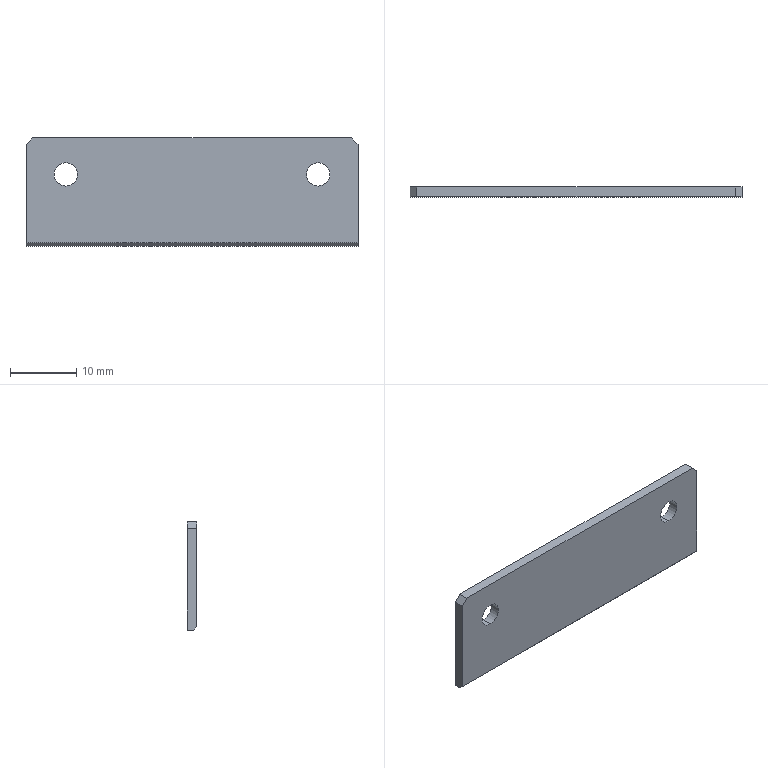Part | SolidWorks | features Chamfer 2, Extrusion 1, ICE 1 | 1 solid | 13 faces | box 50 x 1.5 x 16.3 mm | volume 1186 mm3 | plane 9 | cylinder 4 | commonest cylinder face diameters 3.5 x4
STEP:
#1=CARTESIAN_POINT('',(19.,0.,0.9));
#2=VERTEX_POINT('',#1);
#3=CARTESIAN_POINT('',(19.,0.,4.4));
#4=VERTEX_POINT('',#3);
#5=CARTESIAN_POINT('',(19.,0.,2.65));
#6=DIRECTION('',(0.,1.,0.));
#7=DIRECTION('',(0.,0.,1.));
#8=AXIS2_PLACEMENT_3D('',#5,#6,#7);
#9=CIRCLE('',#8,1.75);
#10=EDGE_CURVE('',#2,#4,#9,.T.);
#11=ORIENTED_EDGE('',*,*,#10,.F.);
#12=CARTESIAN_POINT('',(19.,1.5,0.9));
#13=VERTEX_POINT('',#12);
#14=CARTESIAN_POINT('',(19.,-8.5,0.9));
#15=DIRECTION('',(0.,1.,0.));
#16=VECTOR('',#15,1000.);
#17=LINE('',#14,#16);
#18=EDGE_CURVE('',#2,#13,#17,.T.);
#19=ORIENTED_EDGE('',*,*,#18,.T.);
#20=CARTESIAN_POINT('',(19.,1.5,4.4));
#21=VERTEX_POINT('',#20);
#22=CARTESIAN_POINT('',(19.,1.5,2.65));
#23=DIRECTION('',(0.,1.,0.));
#24=DIRECTION('',(0.,0.,-1.));
#25=AXIS2_PLACEMENT_3D('',#22,#23,#24);
#26=CIRCLE('',#25,1.75);
#27=EDGE_CURVE('',#13,#21,#26,.T.);
#28=ORIENTED_EDGE('',*,*,#27,.T.);
#29=CARTESIAN_POINT('',(19.,-8.5,4.4));
#30=DIRECTION('',(0.,1.,0.));
#31=VECTOR('',#30,1000.);
#32=LINE('',#29,#31);
#33=EDGE_CURVE('',#4,#21,#32,.T.);
#34=ORIENTED_EDGE('',*,*,#33,.F.);
#35=EDGE_LOOP('',(#11,#19,#28,#34));
#36=FACE_OUTER_BOUND('',#35,.T.);
#37=CARTESIAN_POINT('',(19.,-8.5,2.65));
#38=DIRECTION('',(0.,1.,0.));
#39=DIRECTION('',(0.,0.,1.));
#40=AXIS2_PLACEMENT_3D('',#37,#38,#39);
#41=CYLINDRICAL_SURFACE('',#40,1.75);
#42=ADVANCED_FACE('',(#36),#41,.F.);
#43=CARTESIAN_POINT('',(-19.,0.,0.9));
#44=VERTEX_POINT('',#43);
#45=CARTESIAN_POINT('',(-19.,0.,4.4));
#46=VERTEX_POINT('',#45);
#47=CARTESIAN_POINT('',(-19.,0.,2.65));
#48=DIRECTION('',(0.,1.,0.));
#49=DIRECTION('',(0.,0.,1.));
#50=AXIS2_PLACEMENT_3D('',#47,#48,#49);
#51=CIRCLE('',#50,1.75);
#52=EDGE_CURVE('',#44,#46,#51,.T.);
#53=ORIENTED_EDGE('',*,*,#52,.F.);
#54=CARTESIAN_POINT('',(-19.,1.5,0.9));
#55=VERTEX_POINT('',#54);
#56=CARTESIAN_POINT('',(-19.,-8.5,0.9));
#57=DIRECTION('',(0.,1.,0.));
#58=VECTOR('',#57,1000.);
#59=LINE('',#56,#58);
#60=EDGE_CURVE('',#44,#55,#59,.T.);
#61=ORIENTED_EDGE('',*,*,#60,.T.);
#62=CARTESIAN_POINT('',(-19.,1.5,4.4));
#63=VERTEX_POINT('',#62);
#64=CARTESIAN_POINT('',(-19.,1.5,2.65));
#65=DIRECTION('',(0.,1.,0.));
#66=DIRECTION('',(0.,0.,1.));
#67=AXIS2_PLACEMENT_3D('',#64,#65,#66);
#68=CIRCLE('',#67,1.75);
#69=EDGE_CURVE('',#55,#63,#68,.T.);
#70=ORIENTED_EDGE('',*,*,#69,.T.);
#71=CARTESIAN_POINT('',(-19.,-8.5,4.4));
#72=DIRECTION('',(0.,1.,0.));
#73=VECTOR('',#72,1000.);
#74=LINE('',#71,#73);
#75=EDGE_CURVE('',#46,#63,#74,.T.);
#76=ORIENTED_EDGE('',*,*,#75,.F.);
#77=EDGE_LOOP('',(#53,#61,#70,#76));
#78=FACE_OUTER_BOUND('',#77,.T.);
#79=CARTESIAN_POINT('',(-19.,-8.5,2.65));
#80=DIRECTION('',(0.,1.,0.));
#81=DIRECTION('',(0.,0.,1.));
#82=AXIS2_PLACEMENT_3D('',#79,#80,#81);
#83=CYLINDRICAL_SURFACE('',#82,1.75);
#84=ADVANCED_FACE('',(#78),#83,.F.);
#85=CARTESIAN_POINT('',(25.,0.,7.15));
#86=VERTEX_POINT('',#85);
#87=CARTESIAN_POINT('',(25.,0.,-7.65));
#88=VERTEX_POINT('',#87);
#89=CARTESIAN_POINT('',(25.,0.,-8.15));
#90=DIRECTION('',(0.,0.,-1.));
#91=VECTOR('',#90,1000.);
#92=LINE('',#89,#91);
#93=EDGE_CURVE('',#86,#88,#92,.T.);
#94=ORIENTED_EDGE('',*,*,#93,.T.);
#95=CARTESIAN_POINT('',(25.,0.5,-8.15));
#96=VERTEX_POINT('',#95);
#97=CARTESIAN_POINT('',(25.,0.5,-8.15));
#98=DIRECTION('',(0.,0.7071,-0.7071));
#99=VECTOR('',#98,1000.);
#100=LINE('',#97,#99);
#101=EDGE_CURVE('',#88,#96,#100,.T.);
#102=ORIENTED_EDGE('',*,*,#101,.T.);
#103=CARTESIAN_POINT('',(25.,1.5,-8.15));
#104=VERTEX_POINT('',#103);
#105=CARTESIAN_POINT('',(25.,1.5,-8.15));
#106=DIRECTION('',(0.,-1.,0.));
#107=VECTOR('',#106,1000.);
#108=LINE('',#105,#107);
#109=EDGE_CURVE('',#104,#96,#108,.T.);
#110=ORIENTED_EDGE('',*,*,#109,.F.);
#111=CARTESIAN_POINT('',(25.,1.5,7.15));
#112=VERTEX_POINT('',#111);
#113=CARTESIAN_POINT('',(25.,1.5,-8.15));
#114=DIRECTION('',(0.,0.,-1.));
#115=VECTOR('',#114,1000.);
#116=LINE('',#113,#115);
#117=EDGE_CURVE('',#112,#104,#116,.T.);
#118=ORIENTED_EDGE('',*,*,#117,.F.);
#119=CARTESIAN_POINT('',(25.,1.5,7.15));
#120=DIRECTION('',(0.,-1.,0.));
#121=VECTOR('',#120,1000.);
#122=LINE('',#119,#121);
#123=EDGE_CURVE('',#112,#86,#122,.T.);
#124=ORIENTED_EDGE('',*,*,#123,.T.);
#125=EDGE_LOOP('',(#94,#102,#110,#118,#124));
#126=FACE_OUTER_BOUND('',#125,.T.);
#127=CARTESIAN_POINT('',(25.,1.5,-8.15));
#128=DIRECTION('',(-1.,0.,0.));
#129=DIRECTION('',(0.,0.,1.));
#130=AXIS2_PLACEMENT_3D('',#127,#128,#129);
#131=PLANE('',#130);
#132=ADVANCED_FACE('',(#126),#131,.F.);
#133=ORIENTED_EDGE('',*,*,#109,.T.);
#134=CARTESIAN_POINT('',(-25.,0.5,-8.15));
#135=VERTEX_POINT('',#134);
#136=CARTESIAN_POINT('',(-25.,0.5,-8.15));
#137=DIRECTION('',(-1.,0.,0.));
#138=VECTOR('',#137,1000.);
#139=LINE('',#136,#138);
#140=EDGE_CURVE('',#96,#135,#139,.T.);
#141=ORIENTED_EDGE('',*,*,#140,.T.);
#142=CARTESIAN_POINT('',(-25.,1.5,-8.15));
#143=VERTEX_POINT('',#142);
#144=CARTESIAN_POINT('',(-25.,1.5,-8.15));
#145=DIRECTION('',(0.,-1.,0.));
#146=VECTOR('',#145,1000.);
#147=LINE('',#144,#146);
#148=EDGE_CURVE('',#143,#135,#147,.T.);
#149=ORIENTED_EDGE('',*,*,#148,.F.);
#150=CARTESIAN_POINT('',(-25.,1.5,-8.15));
#151=DIRECTION('',(-1.,0.,0.));
#152=VECTOR('',#151,1000.);
#153=LINE('',#150,#152);
#154=EDGE_CURVE('',#104,#143,#153,.T.);
#155=ORIENTED_EDGE('',*,*,#154,.F.);
#156=EDGE_LOOP('',(#133,#141,#149,#155));
#157=FACE_OUTER_BOUND('',#156,.T.);
#158=CARTESIAN_POINT('',(-25.,1.5,-8.15));
#159=DIRECTION('',(0.,0.,1.));
#160=DIRECTION('',(1.,0.,0.));
#161=AXIS2_PLACEMENT_3D('',#158,#159,#160);
#162=PLANE('',#161);
#163=ADVANCED_FACE('',(#157),#162,.F.);
#164=ORIENTED_EDGE('',*,*,#148,.T.);
#165=CARTESIAN_POINT('',(-25.,0.,-7.65));
#166=VERTEX_POINT('',#165);
#167=CARTESIAN_POINT('',(-25.,0.5,-8.15));
#168=DIRECTION('',(0.,-0.7071,0.7071));
#169=VECTOR('',#168,1000.);
#170=LINE('',#167,#169);
#171=EDGE_CURVE('',#135,#166,#170,.T.);
#172=ORIENTED_EDGE('',*,*,#171,.T.);
#173=CARTESIAN_POINT('',(-25.,0.,7.15));
#174=VERTEX_POINT('',#173);
#175=CARTESIAN_POINT('',(-25.,0.,-8.15));
#176=DIRECTION('',(0.,0.,1.));
#177=VECTOR('',#176,1000.);
#178=LINE('',#175,#177);
#179=EDGE_CURVE('',#166,#174,#178,.T.);
#180=ORIENTED_EDGE('',*,*,#179,.T.);
#181=CARTESIAN_POINT('',(-25.,1.5,7.15));
#182=VERTEX_POINT('',#181);
#183=CARTESIAN_POINT('',(-25.,1.5,7.15));
#184=DIRECTION('',(0.,1.,0.));
#185=VECTOR('',#184,1000.);
#186=LINE('',#183,#185);
#187=EDGE_CURVE('',#174,#182,#186,.T.);
#188=ORIENTED_EDGE('',*,*,#187,.T.);
#189=CARTESIAN_POINT('',(-25.,1.5,-8.15));
#190=DIRECTION('',(0.,0.,1.));
#191=VECTOR('',#190,1000.);
#192=LINE('',#189,#191);
#193=EDGE_CURVE('',#143,#182,#192,.T.);
#194=ORIENTED_EDGE('',*,*,#193,.F.);
#195=EDGE_LOOP('',(#164,#172,#180,#188,#194));
#196=FACE_OUTER_BOUND('',#195,.T.);
#197=CARTESIAN_POINT('',(-25.,1.5,-8.15));
#198=DIRECTION('',(1.,0.,0.));
#199=DIRECTION('',(0.,0.,-1.));
#200=AXIS2_PLACEMENT_3D('',#197,#198,#199);
#201=PLANE('',#200);
#202=ADVANCED_FACE('',(#196),#201,.F.);
#203=CARTESIAN_POINT('',(-24.,0.,8.15));
#204=VERTEX_POINT('',#203);
#205=CARTESIAN_POINT('',(24.,0.,8.15));
#206=VERTEX_POINT('',#205);
#207=CARTESIAN_POINT('',(-25.,0.,8.15));
#208=DIRECTION('',(1.,0.,0.));
#209=VECTOR('',#208,1000.);
#210=LINE('',#207,#209);
#211=EDGE_CURVE('',#204,#206,#210,.T.);
#212=ORIENTED_EDGE('',*,*,#211,.T.);
#213=CARTESIAN_POINT('',(24.,1.5,8.15));
#214=VERTEX_POINT('',#213);
#215=CARTESIAN_POINT('',(24.,1.5,8.15));
#216=DIRECTION('',(0.,1.,0.));
#217=VECTOR('',#216,1000.);
#218=LINE('',#215,#217);
#219=EDGE_CURVE('',#206,#214,#218,.T.);
#220=ORIENTED_EDGE('',*,*,#219,.T.);
#221=CARTESIAN_POINT('',(-24.,1.5,8.15));
#222=VERTEX_POINT('',#221);
#223=CARTESIAN_POINT('',(-25.,1.5,8.15));
#224=DIRECTION('',(1.,0.,0.));
#225=VECTOR('',#224,1000.);
#226=LINE('',#223,#225);
#227=EDGE_CURVE('',#222,#214,#226,.T.);
#228=ORIENTED_EDGE('',*,*,#227,.F.);
#229=CARTESIAN_POINT('',(-24.,1.5,8.15));
#230=DIRECTION('',(0.,-1.,0.));
#231=VECTOR('',#230,1000.);
#232=LINE('',#229,#231);
#233=EDGE_CURVE('',#222,#204,#232,.T.);
#234=ORIENTED_EDGE('',*,*,#233,.T.);
#235=EDGE_LOOP('',(#212,#220,#228,#234));
#236=FACE_OUTER_BOUND('',#235,.T.);
#237=CARTESIAN_POINT('',(-25.,1.5,8.15));
#238=DIRECTION('',(0.,0.,-1.));
#239=DIRECTION('',(-1.,0.,0.));
#240=AXIS2_PLACEMENT_3D('',#237,#238,#239);
#241=PLANE('',#240);
#242=ADVANCED_FACE('',(#236),#241,.F.);
#243=CARTESIAN_POINT('',(19.,1.5,2.65));
#244=DIRECTION('',(0.,1.,0.));
#245=DIRECTION('',(0.,0.,-1.));
#246=AXIS2_PLACEMENT_3D('',#243,#244,#245);
#247=CIRCLE('',#246,1.75);
#248=EDGE_CURVE('',#21,#13,#247,.T.);
#249=ORIENTED_EDGE('',*,*,#248,.F.);
#250=ORIENTED_EDGE('',*,*,#27,.F.);
#251=EDGE_LOOP('',(#249,#250));
#252=FACE_BOUND('',#251,.T.);
#253=CARTESIAN_POINT('',(-19.,1.5,2.65));
#254=DIRECTION('',(0.,1.,0.));
#255=DIRECTION('',(0.,0.,1.));
#256=AXIS2_PLACEMENT_3D('',#253,#254,#255);
#257=CIRCLE('',#256,1.75);
#258=EDGE_CURVE('',#63,#55,#257,.T.);
#259=ORIENTED_EDGE('',*,*,#258,.F.);
#260=ORIENTED_EDGE('',*,*,#69,.F.);
#261=EDGE_LOOP('',(#259,#260));
#262=FACE_BOUND('',#261,.T.);
#263=ORIENTED_EDGE('',*,*,#227,.T.);
#264=CARTESIAN_POINT('',(16.075,1.5,16.075));
#265=DIRECTION('',(0.7071,0.,-0.7071));
#266=VECTOR('',#265,1000.);
#267=LINE('',#264,#266);
#268=EDGE_CURVE('',#214,#112,#267,.T.);
#269=ORIENTED_EDGE('',*,*,#268,.T.);
#270=ORIENTED_EDGE('',*,*,#117,.T.);
#271=ORIENTED_EDGE('',*,*,#154,.T.);
#272=ORIENTED_EDGE('',*,*,#193,.T.);
#273=CARTESIAN_POINT('',(-16.075,1.5,16.075));
#274=DIRECTION('',(0.7071,0.,0.7071));
#275=VECTOR('',#274,1000.);
#276=LINE('',#273,#275);
#277=EDGE_CURVE('',#182,#222,#276,.T.);
#278=ORIENTED_EDGE('',*,*,#277,.T.);
#279=EDGE_LOOP('',(#263,#269,#270,#271,#272,#278));
#280=FACE_OUTER_BOUND('',#279,.T.);
#281=CARTESIAN_POINT('',(0.,1.5,0.));
#282=DIRECTION('',(0.,1.,0.));
#283=DIRECTION('',(0.,0.,1.));
#284=AXIS2_PLACEMENT_3D('',#281,#282,#283);
#285=PLANE('',#284);
#286=ADVANCED_FACE('',(#252,#262,#280),#285,.T.);
#287=CARTESIAN_POINT('',(19.,0.,2.65));
#288=DIRECTION('',(0.,1.,0.));
#289=DIRECTION('',(0.,0.,1.));
#290=AXIS2_PLACEMENT_3D('',#287,#288,#289);
#291=CIRCLE('',#290,1.75);
#292=EDGE_CURVE('',#4,#2,#291,.T.);
#293=ORIENTED_EDGE('',*,*,#292,.T.);
#294=ORIENTED_EDGE('',*,*,#10,.T.);
#295=EDGE_LOOP('',(#293,#294));
#296=FACE_BOUND('',#295,.T.);
#297=CARTESIAN_POINT('',(-19.,0.,2.65));
#298=DIRECTION('',(0.,1.,0.));
#299=DIRECTION('',(0.,0.,1.));
#300=AXIS2_PLACEMENT_3D('',#297,#298,#299);
#301=CIRCLE('',#300,1.75);
#302=EDGE_CURVE('',#46,#44,#301,.T.);
#303=ORIENTED_EDGE('',*,*,#302,.T.);
#304=ORIENTED_EDGE('',*,*,#52,.T.);
#305=EDGE_LOOP('',(#303,#304));
#306=FACE_BOUND('',#305,.T.);
#307=ORIENTED_EDGE('',*,*,#179,.F.);
#308=CARTESIAN_POINT('',(0.,0.,-7.65));
#309=DIRECTION('',(1.,0.,0.));
#310=VECTOR('',#309,1000.);
#311=LINE('',#308,#310);
#312=EDGE_CURVE('',#166,#88,#311,.T.);
#313=ORIENTED_EDGE('',*,*,#312,.T.);
#314=ORIENTED_EDGE('',*,*,#93,.F.);
#315=CARTESIAN_POINT('',(25.,0.,7.15));
#316=DIRECTION('',(-0.7071,0.,0.7071));
#317=VECTOR('',#316,1000.);
#318=LINE('',#315,#317);
#319=EDGE_CURVE('',#86,#206,#318,.T.);
#320=ORIENTED_EDGE('',*,*,#319,.T.);
#321=ORIENTED_EDGE('',*,*,#211,.F.);
#322=CARTESIAN_POINT('',(-24.,0.,8.15));
#323=DIRECTION('',(-0.7071,0.,-0.7071));
#324=VECTOR('',#323,1000.);
#325=LINE('',#322,#324);
#326=EDGE_CURVE('',#204,#174,#325,.T.);
#327=ORIENTED_EDGE('',*,*,#326,.T.);
#328=EDGE_LOOP('',(#307,#313,#314,#320,#321,#327));
#329=FACE_OUTER_BOUND('',#328,.T.);
#330=CARTESIAN_POINT('',(0.,0.,0.));
#331=DIRECTION('',(0.,1.,0.));
#332=DIRECTION('',(0.,0.,1.));
#333=AXIS2_PLACEMENT_3D('',#330,#331,#332);
#334=PLANE('',#333);
#335=ADVANCED_FACE('',(#296,#306,#329),#334,.F.);
#336=ORIENTED_EDGE('',*,*,#60,.F.);
#337=ORIENTED_EDGE('',*,*,#302,.F.);
#338=ORIENTED_EDGE('',*,*,#75,.T.);
#339=ORIENTED_EDGE('',*,*,#258,.T.);
#340=EDGE_LOOP('',(#336,#337,#338,#339));
#341=FACE_OUTER_BOUND('',#340,.T.);
#342=CARTESIAN_POINT('',(-19.,-8.5,2.65));
#343=DIRECTION('',(0.,1.,0.));
#344=DIRECTION('',(0.,0.,1.));
#345=AXIS2_PLACEMENT_3D('',#342,#343,#344);
#346=CYLINDRICAL_SURFACE('',#345,1.75);
#347=ADVANCED_FACE('',(#341),#346,.F.);
#348=ORIENTED_EDGE('',*,*,#18,.F.);
#349=ORIENTED_EDGE('',*,*,#292,.F.);
#350=ORIENTED_EDGE('',*,*,#33,.T.);
#351=ORIENTED_EDGE('',*,*,#248,.T.);
#352=EDGE_LOOP('',(#348,#349,#350,#351));
#353=FACE_OUTER_BOUND('',#352,.T.);
#354=CARTESIAN_POINT('',(19.,-8.5,2.65));
#355=DIRECTION('',(0.,1.,0.));
#356=DIRECTION('',(0.,0.,1.));
#357=AXIS2_PLACEMENT_3D('',#354,#355,#356);
#358=CYLINDRICAL_SURFACE('',#357,1.75);
#359=ADVANCED_FACE('',(#353),#358,.F.);
#360=ORIENTED_EDGE('',*,*,#268,.F.);
#361=ORIENTED_EDGE('',*,*,#219,.F.);
#362=ORIENTED_EDGE('',*,*,#319,.F.);
#363=ORIENTED_EDGE('',*,*,#123,.F.);
#364=EDGE_LOOP('',(#360,#361,#362,#363));
#365=FACE_OUTER_BOUND('',#364,.T.);
#366=CARTESIAN_POINT('',(25.,1.5,7.15));
#367=DIRECTION('',(-0.7071,0.,-0.7071));
#368=DIRECTION('',(0.,-1.,0.));
#369=AXIS2_PLACEMENT_3D('',#366,#367,#368);
#370=PLANE('',#369);
#371=ADVANCED_FACE('',(#365),#370,.F.);
#372=ORIENTED_EDGE('',*,*,#277,.F.);
#373=ORIENTED_EDGE('',*,*,#187,.F.);
#374=ORIENTED_EDGE('',*,*,#326,.F.);
#375=ORIENTED_EDGE('',*,*,#233,.F.);
#376=EDGE_LOOP('',(#372,#373,#374,#375));
#377=FACE_OUTER_BOUND('',#376,.T.);
#378=CARTESIAN_POINT('',(-24.,1.5,8.15));
#379=DIRECTION('',(0.7071,0.,-0.7071));
#380=DIRECTION('',(0.,-1.,0.));
#381=AXIS2_PLACEMENT_3D('',#378,#379,#380);
#382=PLANE('',#381);
#383=ADVANCED_FACE('',(#377),#382,.F.);
#384=ORIENTED_EDGE('',*,*,#101,.F.);
#385=ORIENTED_EDGE('',*,*,#312,.F.);
#386=ORIENTED_EDGE('',*,*,#171,.F.);
#387=ORIENTED_EDGE('',*,*,#140,.F.);
#388=EDGE_LOOP('',(#384,#385,#386,#387));
#389=FACE_OUTER_BOUND('',#388,.T.);
#390=CARTESIAN_POINT('',(-25.,0.5,-8.15));
#391=DIRECTION('',(0.,0.7071,0.7071));
#392=DIRECTION('',(-1.,0.,0.));
#393=AXIS2_PLACEMENT_3D('',#390,#391,#392);
#394=PLANE('',#393);
#395=ADVANCED_FACE('',(#389),#394,.F.);
#396=CLOSED_SHELL('',(#42,#84,#132,#163,#202,#242,#286,#335,#347,#359,#371,#383,#395));
#397=MANIFOLD_SOLID_BREP('',#396);
#398=CARTESIAN_POINT('',(0.,0.,0.));
#399=DIRECTION('',(0.,0.,1.));
#400=DIRECTION('',(1.,0.,0.));
#401=AXIS2_PLACEMENT_3D('',#398,#399,#400);
#402=(LENGTH_UNIT()NAMED_UNIT(*)SI_UNIT(.MILLI.,.METRE.));
#403=UNCERTAINTY_MEASURE_WITH_UNIT(LENGTH_MEASURE(0.00001),#402,'','');
#404=(NAMED_UNIT(*)PLANE_ANGLE_UNIT()SI_UNIT($,.RADIAN.));
#405=(NAMED_UNIT(*)SI_UNIT($,.STERADIAN.)SOLID_ANGLE_UNIT());
#406=(GEOMETRIC_REPRESENTATION_CONTEXT(3)GLOBAL_UNCERTAINTY_ASSIGNED_CONTEXT((#403))GLOBAL_UNIT_ASSIGNED_CONTEXT((#402,#404,#405))REPRESENTATION_CONTEXT('',''));
#407=ADVANCED_BREP_SHAPE_REPRESENTATION('',(#397,#401),#406);